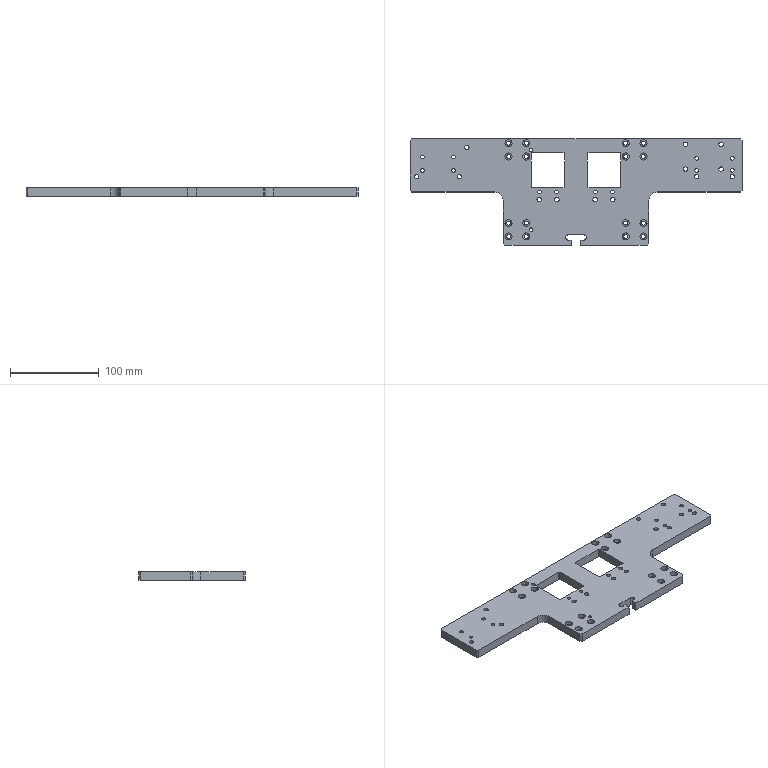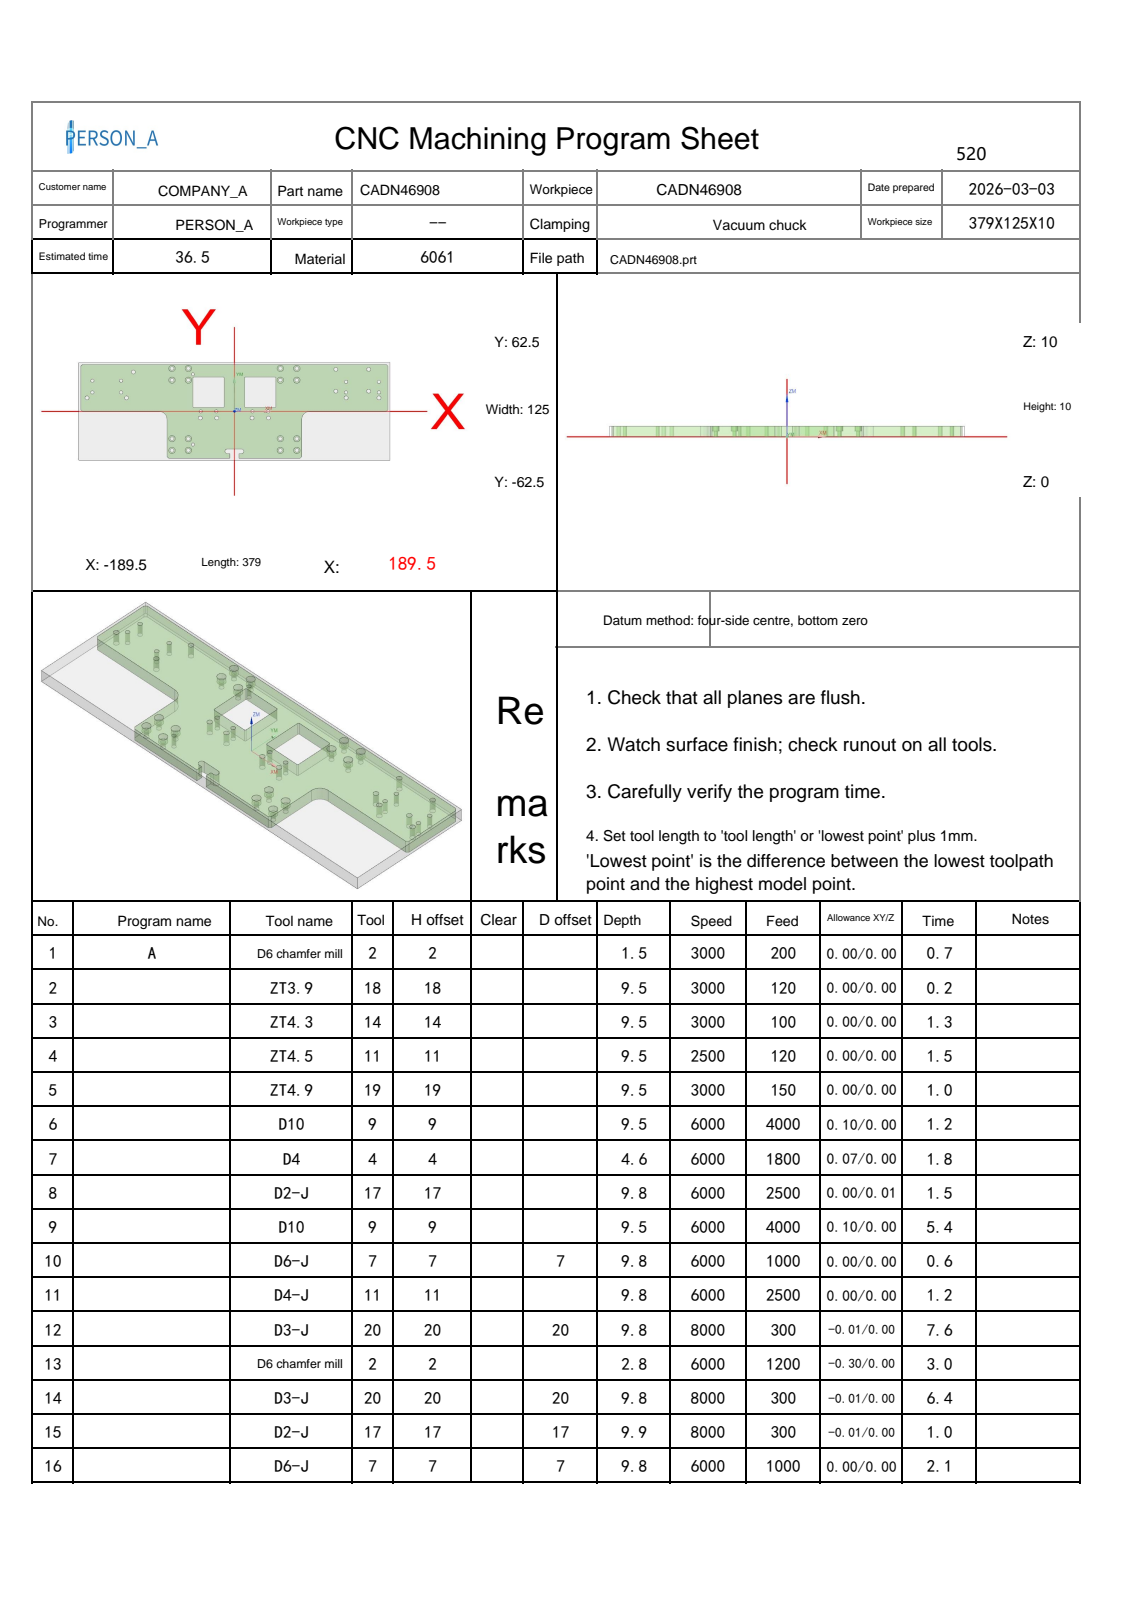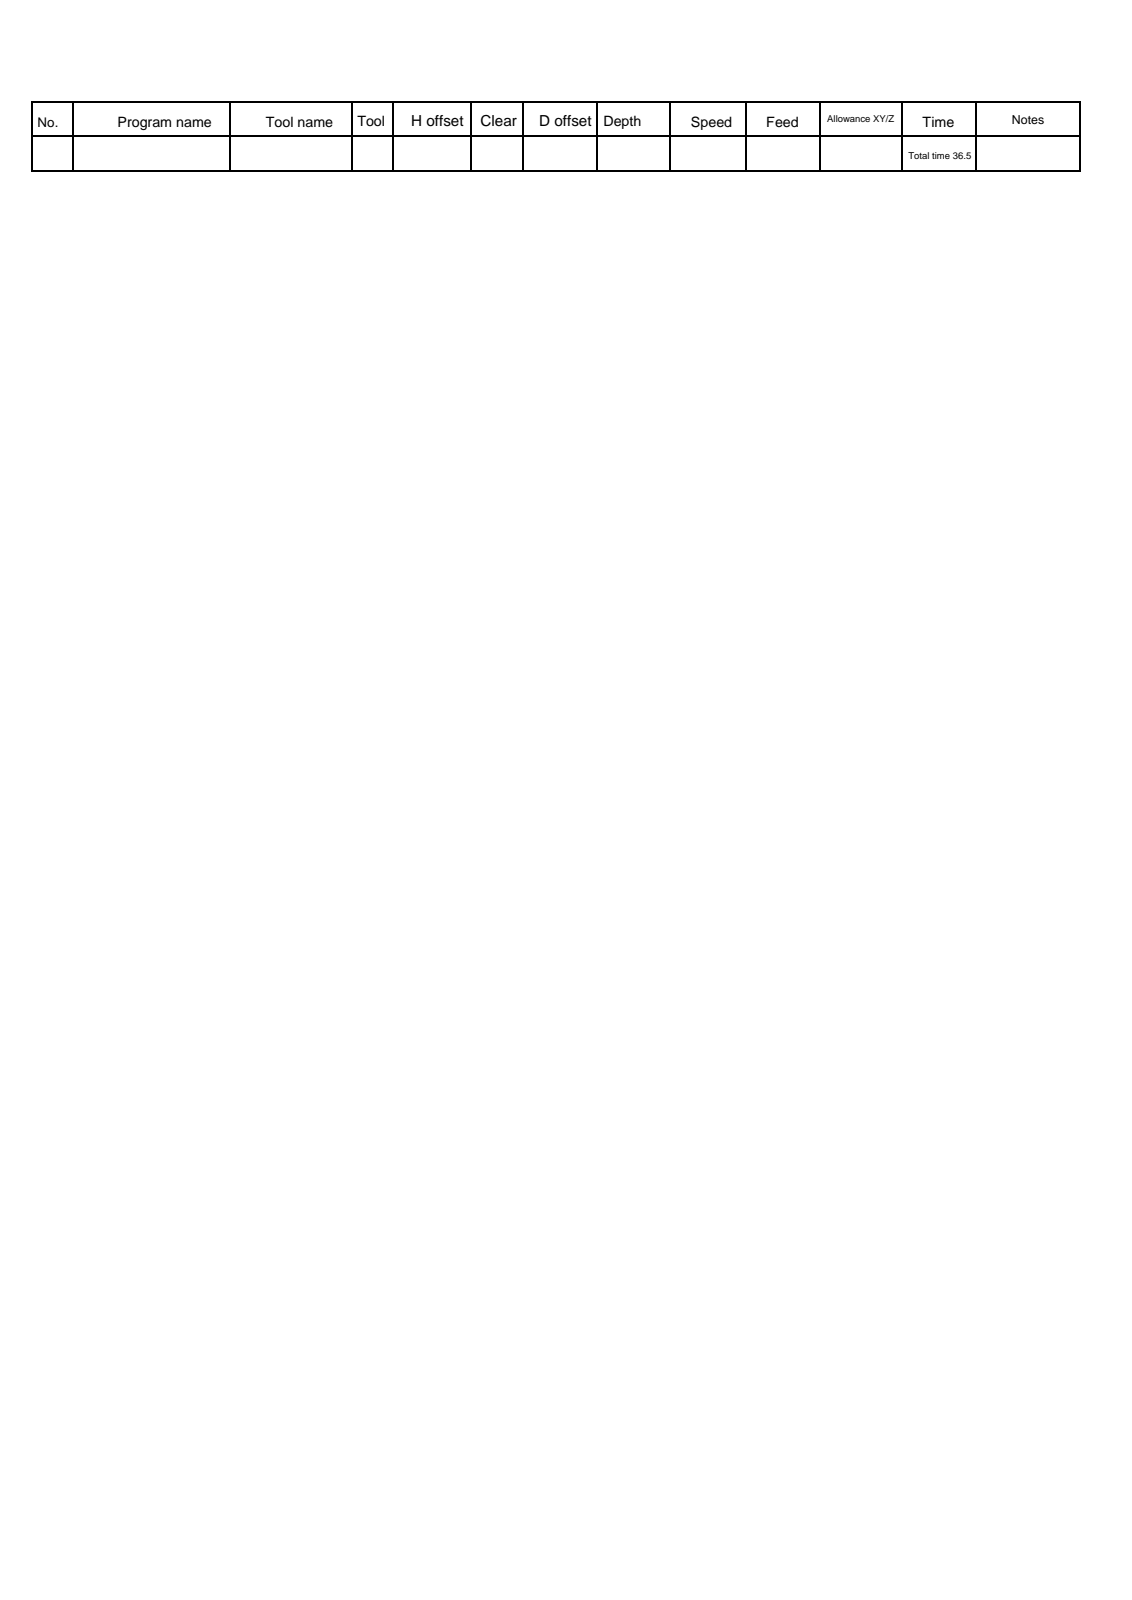NC program | NX | posted by the shop | part box 374 x 120 x 10 mm
Lines 6179 to 7020 of 15301:
N9 T09 M06
(D10  D=10. R=0. H=09 ce=0.10 di=0.00)
G00 G90 G54 X0.0 Y65.1 M03 S6000
G43 H09 Z40.
M08
Z10.5
G01 X185. Z10.41 F4000.
G02 X188.606 Y63.606 Z10.408 I0.0 J-5.1
G01 X190.606 Y61.606 Z10.406
G02 X192.1 Y58. Z10.404 I-3.606 J-3.606
G01 Y2. Z10.377
G02 X190.606 Y-1.606 Z10.375 I-5.1 J0.0
G01 X188.606 Y-3.606 Z10.374
G02 X185. Y-5.1 Z10.372 I-3.606 J3.606
G01 X92. Z10.326
G03 X87.1 Y-10. Z10.323 I0.0 J-4.9
G01 Y-58. Z10.299
G02 X85.606 Y-61.606 Z10.297 I-5.1 J0.0
G01 X83.606 Y-63.606 Z10.296
G02 X80. Y-65.1 Z10.294 I-3.606 J3.606
G01 X5.5 Z10.257
G02 X.4 Y-60. Z10.254 I0.0 J5.1
G01 Y-54.2 Z10.251
G02 X.48 Y-53.3 Z10.25 I5.1 J0.0
G01 X-.48
G02 X-.4 Y-54.2 Z10.249 I-5.02 J-.9
G01 Y-60. Z10.246
G02 X-5.5 Y-65.1 Z10.243 I-5.1 J0.0
G01 X-80. Z10.206
G02 X-83.606 Y-63.606 Z10.204 I0.0 J5.1
G01 X-85.606 Y-61.606 Z10.203
G02 X-87.1 Y-58. Z10.201 I3.606 J3.606
G01 Y-10. Z10.177
G03 X-92. Y-5.1 Z10.174 I-4.9 J0.0
G01 X-185. Z10.128
G02 X-188.606 Y-3.606 Z10.126 I0.0 J5.1
G01 X-190.606 Y-1.606 Z10.125
G02 X-192.1 Y2. Z10.123 I3.606 J3.606
G01 Y58. Z10.096
G02 X-190.606 Y61.606 Z10.094 I5.1 J0.0
G01 X-188.606 Y63.606 Z10.092
G02 X-185. Y65.1 Z10.09 I3.606 J-3.606
G01 X185. Z9.91
G02 X188.606 Y63.606 Z9.908 I0.0 J-5.1
G01 X190.606 Y61.606 Z9.906
G02 X192.1 Y58. Z9.904 I-3.606 J-3.606
G01 Y2. Z9.877
G02 X190.606 Y-1.606 Z9.875 I-5.1 J0.0
G01 X188.606 Y-3.606 Z9.874
G02 X185. Y-5.1 Z9.872 I-3.606 J3.606
G01 X92. Z9.826
G03 X87.1 Y-10. Z9.823 I0.0 J-4.9
G01 Y-58. Z9.799
G02 X85.606 Y-61.606 Z9.797 I-5.1 J0.0
G01 X83.606 Y-63.606 Z9.796
G02 X80. Y-65.1 Z9.794 I-3.606 J3.606
G01 X5.5 Z9.757
G02 X.4 Y-60. Z9.754 I0.0 J5.1
G01 Y-54.2 Z9.751
G02 X.48 Y-53.3 Z9.75 I5.1 J0.0
G01 X-.48
G02 X-.4 Y-54.2 Z9.749 I-5.02 J-.9
G01 Y-60. Z9.746
G02 X-5.5 Y-65.1 Z9.743 I-5.1 J0.0
G01 X-80. Z9.706
G02 X-83.606 Y-63.606 Z9.704 I0.0 J5.1
G01 X-85.606 Y-61.606 Z9.703
G02 X-87.1 Y-58. Z9.701 I3.606 J3.606
G01 Y-10. Z9.677
G03 X-92. Y-5.1 Z9.674 I-4.9 J0.0
G01 X-185. Z9.628
G02 X-188.606 Y-3.606 Z9.626 I0.0 J5.1
G01 X-190.606 Y-1.606 Z9.625
G02 X-192.1 Y2. Z9.623 I3.606 J3.606
G01 Y58. Z9.596
G02 X-190.606 Y61.606 Z9.594 I5.1 J0.0
G01 X-188.606 Y63.606 Z9.592
G02 X-185. Y65.1 Z9.59 I3.606 J-3.606
G01 X185. Z9.41
G02 X188.606 Y63.606 Z9.408 I0.0 J-5.1
G01 X190.606 Y61.606 Z9.406
G02 X192.1 Y58. Z9.404 I-3.606 J-3.606
G01 Y2. Z9.377
G02 X190.606 Y-1.606 Z9.375 I-5.1 J0.0
G01 X188.606 Y-3.606 Z9.374
G02 X185. Y-5.1 Z9.372 I-3.606 J3.606
G01 X92. Z9.326
G03 X87.1 Y-10. Z9.323 I0.0 J-4.9
G01 Y-58. Z9.299
G02 X85.606 Y-61.606 Z9.297 I-5.1 J0.0
G01 X83.606 Y-63.606 Z9.296
G02 X80. Y-65.1 Z9.294 I-3.606 J3.606
G01 X5.5 Z9.257
G02 X.4 Y-60. Z9.254 I0.0 J5.1
G01 Y-54.2 Z9.251
G02 X.48 Y-53.3 Z9.25 I5.1 J0.0
G01 X-.48
G02 X-.4 Y-54.2 Z9.249 I-5.02 J-.9
G01 Y-60. Z9.246
G02 X-5.5 Y-65.1 Z9.243 I-5.1 J0.0
G01 X-80. Z9.206
G02 X-83.606 Y-63.606 Z9.204 I0.0 J5.1
G01 X-85.606 Y-61.606 Z9.203
G02 X-87.1 Y-58. Z9.201 I3.606 J3.606
G01 Y-10. Z9.177
G03 X-92. Y-5.1 Z9.174 I-4.9 J0.0
G01 X-185. Z9.128
G02 X-188.606 Y-3.606 Z9.126 I0.0 J5.1
G01 X-190.606 Y-1.606 Z9.125
G02 X-192.1 Y2. Z9.123 I3.606 J3.606
G01 Y58. Z9.096
G02 X-190.606 Y61.606 Z9.094 I5.1 J0.0
G01 X-188.606 Y63.606 Z9.092
G02 X-185. Y65.1 Z9.09 I3.606 J-3.606
G01 X185. Z8.91
G02 X188.606 Y63.606 Z8.908 I0.0 J-5.1
G01 X190.606 Y61.606 Z8.906
G02 X192.1 Y58. Z8.904 I-3.606 J-3.606
G01 Y2. Z8.877
G02 X190.606 Y-1.606 Z8.875 I-5.1 J0.0
G01 X188.606 Y-3.606 Z8.874
G02 X185. Y-5.1 Z8.872 I-3.606 J3.606
G01 X92. Z8.826
G03 X87.1 Y-10. Z8.823 I0.0 J-4.9
G01 Y-58. Z8.799
G02 X85.606 Y-61.606 Z8.797 I-5.1 J0.0
G01 X83.606 Y-63.606 Z8.796
G02 X80. Y-65.1 Z8.794 I-3.606 J3.606
G01 X5.5 Z8.757
G02 X.4 Y-60. Z8.754 I0.0 J5.1
G01 Y-54.2 Z8.751
G02 X.48 Y-53.3 Z8.75 I5.1 J0.0
G01 X-.48
G02 X-.4 Y-54.2 Z8.749 I-5.02 J-.9
G01 Y-60. Z8.746
G02 X-5.5 Y-65.1 Z8.743 I-5.1 J0.0
G01 X-80. Z8.706
G02 X-83.606 Y-63.606 Z8.704 I0.0 J5.1
G01 X-85.606 Y-61.606 Z8.703
G02 X-87.1 Y-58. Z8.701 I3.606 J3.606
G01 Y-10. Z8.677
G03 X-92. Y-5.1 Z8.674 I-4.9 J0.0
G01 X-185. Z8.628
G02 X-188.606 Y-3.606 Z8.626 I0.0 J5.1
G01 X-190.606 Y-1.606 Z8.625
G02 X-192.1 Y2. Z8.623 I3.606 J3.606
G01 Y58. Z8.596
G02 X-190.606 Y61.606 Z8.594 I5.1 J0.0
G01 X-188.606 Y63.606 Z8.592
G02 X-185. Y65.1 Z8.59 I3.606 J-3.606
G01 X185. Z8.41
G02 X188.606 Y63.606 Z8.408 I0.0 J-5.1
G01 X190.606 Y61.606 Z8.406
G02 X192.1 Y58. Z8.404 I-3.606 J-3.606
G01 Y2. Z8.377
G02 X190.606 Y-1.606 Z8.375 I-5.1 J0.0
G01 X188.606 Y-3.606 Z8.374
G02 X185. Y-5.1 Z8.372 I-3.606 J3.606
G01 X92. Z8.326
G03 X87.1 Y-10. Z8.323 I0.0 J-4.9
G01 Y-58. Z8.299
G02 X85.606 Y-61.606 Z8.297 I-5.1 J0.0
G01 X83.606 Y-63.606 Z8.296
G02 X80. Y-65.1 Z8.294 I-3.606 J3.606
G01 X5.5 Z8.257
G02 X.4 Y-60. Z8.254 I0.0 J5.1
G01 Y-54.2 Z8.251
G02 X.48 Y-53.3 Z8.25 I5.1 J0.0
G01 X-.48
G02 X-.4 Y-54.2 Z8.249 I-5.02 J-.9
G01 Y-60. Z8.246
G02 X-5.5 Y-65.1 Z8.243 I-5.1 J0.0
G01 X-80. Z8.206
G02 X-83.606 Y-63.606 Z8.204 I0.0 J5.1
G01 X-85.606 Y-61.606 Z8.203
G02 X-87.1 Y-58. Z8.201 I3.606 J3.606
G01 Y-10. Z8.177
G03 X-92. Y-5.1 Z8.174 I-4.9 J0.0
G01 X-185. Z8.128
G02 X-188.606 Y-3.606 Z8.126 I0.0 J5.1
G01 X-190.606 Y-1.606 Z8.125
G02 X-192.1 Y2. Z8.123 I3.606 J3.606
G01 Y58. Z8.096
G02 X-190.606 Y61.606 Z8.094 I5.1 J0.0
G01 X-188.606 Y63.606 Z8.092
G02 X-185. Y65.1 Z8.09 I3.606 J-3.606
G01 X185. Z7.91
G02 X188.606 Y63.606 Z7.908 I0.0 J-5.1
G01 X190.606 Y61.606 Z7.906
G02 X192.1 Y58. Z7.904 I-3.606 J-3.606
G01 Y2. Z7.877
G02 X190.606 Y-1.606 Z7.875 I-5.1 J0.0
G01 X188.606 Y-3.606 Z7.874
G02 X185. Y-5.1 Z7.872 I-3.606 J3.606
G01 X92. Z7.826
G03 X87.1 Y-10. Z7.823 I0.0 J-4.9
G01 Y-58. Z7.799
G02 X85.606 Y-61.606 Z7.797 I-5.1 J0.0
G01 X83.606 Y-63.606 Z7.796
G02 X80. Y-65.1 Z7.794 I-3.606 J3.606
G01 X5.5 Z7.757
G02 X.4 Y-60. Z7.754 I0.0 J5.1
G01 Y-54.2 Z7.751
G02 X.48 Y-53.3 Z7.75 I5.1 J0.0
G01 X-.48
G02 X-.4 Y-54.2 Z7.749 I-5.02 J-.9
G01 Y-60. Z7.746
G02 X-5.5 Y-65.1 Z7.743 I-5.1 J0.0
G01 X-80. Z7.706
G02 X-83.606 Y-63.606 Z7.704 I0.0 J5.1
G01 X-85.606 Y-61.606 Z7.703
G02 X-87.1 Y-58. Z7.701 I3.606 J3.606
G01 Y-10. Z7.677
G03 X-92. Y-5.1 Z7.674 I-4.9 J0.0
G01 X-185. Z7.628
G02 X-188.606 Y-3.606 Z7.626 I0.0 J5.1
G01 X-190.606 Y-1.606 Z7.625
G02 X-192.1 Y2. Z7.623 I3.606 J3.606
G01 Y58. Z7.596
G02 X-190.606 Y61.606 Z7.594 I5.1 J0.0
G01 X-188.606 Y63.606 Z7.592
G02 X-185. Y65.1 Z7.59 I3.606 J-3.606
G01 X185. Z7.41
G02 X188.606 Y63.606 Z7.408 I0.0 J-5.1
G01 X190.606 Y61.606 Z7.406
G02 X192.1 Y58. Z7.404 I-3.606 J-3.606
G01 Y2. Z7.377
G02 X190.606 Y-1.606 Z7.375 I-5.1 J0.0
G01 X188.606 Y-3.606 Z7.374
G02 X185. Y-5.1 Z7.372 I-3.606 J3.606
G01 X92. Z7.326
G03 X87.1 Y-10. Z7.323 I0.0 J-4.9
G01 Y-58. Z7.299
G02 X85.606 Y-61.606 Z7.297 I-5.1 J0.0
G01 X83.606 Y-63.606 Z7.296
G02 X80. Y-65.1 Z7.294 I-3.606 J3.606
G01 X5.5 Z7.257
G02 X.4 Y-60. Z7.254 I0.0 J5.1
G01 Y-54.2 Z7.251
G02 X.48 Y-53.3 Z7.25 I5.1 J0.0
G01 X-.48
G02 X-.4 Y-54.2 Z7.249 I-5.02 J-.9
G01 Y-60. Z7.246
G02 X-5.5 Y-65.1 Z7.243 I-5.1 J0.0
G01 X-80. Z7.206
G02 X-83.606 Y-63.606 Z7.204 I0.0 J5.1
G01 X-85.606 Y-61.606 Z7.203
G02 X-87.1 Y-58. Z7.201 I3.606 J3.606
G01 Y-10. Z7.177
G03 X-92. Y-5.1 Z7.174 I-4.9 J0.0
G01 X-185. Z7.128
G02 X-188.606 Y-3.606 Z7.126 I0.0 J5.1
G01 X-190.606 Y-1.606 Z7.125
G02 X-192.1 Y2. Z7.123 I3.606 J3.606
G01 Y58. Z7.096
G02 X-190.606 Y61.606 Z7.094 I5.1 J0.0
G01 X-188.606 Y63.606 Z7.092
G02 X-185. Y65.1 Z7.09 I3.606 J-3.606
G01 X185. Z6.91
G02 X188.606 Y63.606 Z6.908 I0.0 J-5.1
G01 X190.606 Y61.606 Z6.906
G02 X192.1 Y58. Z6.904 I-3.606 J-3.606
G01 Y2. Z6.877
G02 X190.606 Y-1.606 Z6.875 I-5.1 J0.0
G01 X188.606 Y-3.606 Z6.874
G02 X185. Y-5.1 Z6.872 I-3.606 J3.606
G01 X92. Z6.826
G03 X87.1 Y-10. Z6.823 I0.0 J-4.9
G01 Y-58. Z6.799
G02 X85.606 Y-61.606 Z6.797 I-5.1 J0.0
G01 X83.606 Y-63.606 Z6.796
G02 X80. Y-65.1 Z6.794 I-3.606 J3.606
G01 X5.5 Z6.757
G02 X.4 Y-60. Z6.754 I0.0 J5.1
G01 Y-54.2 Z6.751
G02 X.48 Y-53.3 Z6.75 I5.1 J0.0
G01 X-.48
G02 X-.4 Y-54.2 Z6.749 I-5.02 J-.9
G01 Y-60. Z6.746
G02 X-5.5 Y-65.1 Z6.743 I-5.1 J0.0
G01 X-80. Z6.706
G02 X-83.606 Y-63.606 Z6.704 I0.0 J5.1
G01 X-85.606 Y-61.606 Z6.703
G02 X-87.1 Y-58. Z6.701 I3.606 J3.606
G01 Y-10. Z6.677
G03 X-92. Y-5.1 Z6.674 I-4.9 J0.0
G01 X-185. Z6.628
G02 X-188.606 Y-3.606 Z6.626 I0.0 J5.1
G01 X-190.606 Y-1.606 Z6.625
G02 X-192.1 Y2. Z6.623 I3.606 J3.606
G01 Y58. Z6.596
G02 X-190.606 Y61.606 Z6.594 I5.1 J0.0
G01 X-188.606 Y63.606 Z6.592
G02 X-185. Y65.1 Z6.59 I3.606 J-3.606
G01 X185. Z6.41
G02 X188.606 Y63.606 Z6.408 I0.0 J-5.1
G01 X190.606 Y61.606 Z6.406
G02 X192.1 Y58. Z6.404 I-3.606 J-3.606
G01 Y2. Z6.377
G02 X190.606 Y-1.606 Z6.375 I-5.1 J0.0
G01 X188.606 Y-3.606 Z6.374
G02 X185. Y-5.1 Z6.372 I-3.606 J3.606
G01 X92. Z6.326
G03 X87.1 Y-10. Z6.323 I0.0 J-4.9
G01 Y-58. Z6.299
G02 X85.606 Y-61.606 Z6.297 I-5.1 J0.0
G01 X83.606 Y-63.606 Z6.296
G02 X80. Y-65.1 Z6.294 I-3.606 J3.606
G01 X5.5 Z6.257
G02 X.4 Y-60. Z6.254 I0.0 J5.1
G01 Y-54.2 Z6.251
G02 X.48 Y-53.3 Z6.25 I5.1 J0.0
G01 X-.48
G02 X-.4 Y-54.2 Z6.249 I-5.02 J-.9
G01 Y-60. Z6.246
G02 X-5.5 Y-65.1 Z6.243 I-5.1 J0.0
G01 X-80. Z6.206
G02 X-83.606 Y-63.606 Z6.204 I0.0 J5.1
G01 X-85.606 Y-61.606 Z6.203
G02 X-87.1 Y-58. Z6.201 I3.606 J3.606
G01 Y-10. Z6.177
G03 X-92. Y-5.1 Z6.174 I-4.9 J0.0
G01 X-185. Z6.128
G02 X-188.606 Y-3.606 Z6.126 I0.0 J5.1
G01 X-190.606 Y-1.606 Z6.125
G02 X-192.1 Y2. Z6.123 I3.606 J3.606
G01 Y58. Z6.096
G02 X-190.606 Y61.606 Z6.094 I5.1 J0.0
G01 X-188.606 Y63.606 Z6.092
G02 X-185. Y65.1 Z6.09 I3.606 J-3.606
G01 X185. Z5.91
G02 X188.606 Y63.606 Z5.908 I0.0 J-5.1
G01 X190.606 Y61.606 Z5.906
G02 X192.1 Y58. Z5.904 I-3.606 J-3.606
G01 Y2. Z5.877
G02 X190.606 Y-1.606 Z5.875 I-5.1 J0.0
G01 X188.606 Y-3.606 Z5.874
G02 X185. Y-5.1 Z5.872 I-3.606 J3.606
G01 X92. Z5.826
G03 X87.1 Y-10. Z5.823 I0.0 J-4.9
G01 Y-58. Z5.799
G02 X85.606 Y-61.606 Z5.797 I-5.1 J0.0
G01 X83.606 Y-63.606 Z5.796
G02 X80. Y-65.1 Z5.794 I-3.606 J3.606
G01 X5.5 Z5.757
G02 X.4 Y-60. Z5.754 I0.0 J5.1
G01 Y-54.2 Z5.751
G02 X.48 Y-53.3 Z5.75 I5.1 J0.0
G01 X-.48
G02 X-.4 Y-54.2 Z5.749 I-5.02 J-.9
G01 Y-60. Z5.746
G02 X-5.5 Y-65.1 Z5.743 I-5.1 J0.0
G01 X-80. Z5.706
G02 X-83.606 Y-63.606 Z5.704 I0.0 J5.1
G01 X-85.606 Y-61.606 Z5.703
G02 X-87.1 Y-58. Z5.701 I3.606 J3.606
G01 Y-10. Z5.677
G03 X-92. Y-5.1 Z5.674 I-4.9 J0.0
G01 X-185. Z5.628
G02 X-188.606 Y-3.606 Z5.626 I0.0 J5.1
G01 X-190.606 Y-1.606 Z5.625
G02 X-192.1 Y2. Z5.623 I3.606 J3.606
G01 Y58. Z5.596
G02 X-190.606 Y61.606 Z5.594 I5.1 J0.0
G01 X-188.606 Y63.606 Z5.592
G02 X-185. Y65.1 Z5.59 I3.606 J-3.606
G01 X185. Z5.41
G02 X188.606 Y63.606 Z5.408 I0.0 J-5.1
G01 X190.606 Y61.606 Z5.406
G02 X192.1 Y58. Z5.404 I-3.606 J-3.606
G01 Y2. Z5.377
G02 X190.606 Y-1.606 Z5.375 I-5.1 J0.0
G01 X188.606 Y-3.606 Z5.374
G02 X185. Y-5.1 Z5.372 I-3.606 J3.606
G01 X92. Z5.326
G03 X87.1 Y-10. Z5.323 I0.0 J-4.9
G01 Y-58. Z5.299
G02 X85.606 Y-61.606 Z5.297 I-5.1 J0.0
G01 X83.606 Y-63.606 Z5.296
G02 X80. Y-65.1 Z5.294 I-3.606 J3.606
G01 X5.5 Z5.257
G02 X.4 Y-60. Z5.254 I0.0 J5.1
G01 Y-54.2 Z5.251
G02 X.48 Y-53.3 Z5.25 I5.1 J0.0
G01 X-.48
G02 X-.4 Y-54.2 Z5.249 I-5.02 J-.9
G01 Y-60. Z5.246
G02 X-5.5 Y-65.1 Z5.243 I-5.1 J0.0
G01 X-80. Z5.206
G02 X-83.606 Y-63.606 Z5.204 I0.0 J5.1
G01 X-85.606 Y-61.606 Z5.203
G02 X-87.1 Y-58. Z5.201 I3.606 J3.606
G01 Y-10. Z5.177
G03 X-92. Y-5.1 Z5.174 I-4.9 J0.0
G01 X-185. Z5.128
G02 X-188.606 Y-3.606 Z5.126 I0.0 J5.1
G01 X-190.606 Y-1.606 Z5.125
G02 X-192.1 Y2. Z5.123 I3.606 J3.606
G01 Y58. Z5.096
G02 X-190.606 Y61.606 Z5.094 I5.1 J0.0
G01 X-188.606 Y63.606 Z5.092
G02 X-185. Y65.1 Z5.09 I3.606 J-3.606
G01 X185. Z4.91
G02 X188.606 Y63.606 Z4.908 I0.0 J-5.1
G01 X190.606 Y61.606 Z4.906
G02 X192.1 Y58. Z4.904 I-3.606 J-3.606
G01 Y2. Z4.877
G02 X190.606 Y-1.606 Z4.875 I-5.1 J0.0
G01 X188.606 Y-3.606 Z4.874
G02 X185. Y-5.1 Z4.872 I-3.606 J3.606
G01 X92. Z4.826
G03 X87.1 Y-10. Z4.823 I0.0 J-4.9
G01 Y-58. Z4.799
G02 X85.606 Y-61.606 Z4.797 I-5.1 J0.0
G01 X83.606 Y-63.606 Z4.796
G02 X80. Y-65.1 Z4.794 I-3.606 J3.606
G01 X5.5 Z4.757
G02 X.4 Y-60. Z4.754 I0.0 J5.1
G01 Y-54.2 Z4.751
G02 X.48 Y-53.3 Z4.75 I5.1 J0.0
G01 X-.48
G02 X-.4 Y-54.2 Z4.749 I-5.02 J-.9
G01 Y-60. Z4.746
G02 X-5.5 Y-65.1 Z4.743 I-5.1 J0.0
G01 X-80. Z4.706
G02 X-83.606 Y-63.606 Z4.704 I0.0 J5.1
G01 X-85.606 Y-61.606 Z4.703
G02 X-87.1 Y-58. Z4.701 I3.606 J3.606
G01 Y-10. Z4.677
G03 X-92. Y-5.1 Z4.674 I-4.9 J0.0
G01 X-185. Z4.628
G02 X-188.606 Y-3.606 Z4.626 I0.0 J5.1
G01 X-190.606 Y-1.606 Z4.625
G02 X-192.1 Y2. Z4.623 I3.606 J3.606
G01 Y58. Z4.596
G02 X-190.606 Y61.606 Z4.594 I5.1 J0.0
G01 X-188.606 Y63.606 Z4.592
G02 X-185. Y65.1 Z4.59 I3.606 J-3.606
G01 X185. Z4.41
G02 X188.606 Y63.606 Z4.408 I0.0 J-5.1
G01 X190.606 Y61.606 Z4.406
G02 X192.1 Y58. Z4.404 I-3.606 J-3.606
G01 Y2. Z4.377
G02 X190.606 Y-1.606 Z4.375 I-5.1 J0.0
G01 X188.606 Y-3.606 Z4.374
G02 X185. Y-5.1 Z4.372 I-3.606 J3.606
G01 X92. Z4.326
G03 X87.1 Y-10. Z4.323 I0.0 J-4.9
G01 Y-58. Z4.299
G02 X85.606 Y-61.606 Z4.297 I-5.1 J0.0
G01 X83.606 Y-63.606 Z4.296
G02 X80. Y-65.1 Z4.294 I-3.606 J3.606
G01 X5.5 Z4.257
G02 X.4 Y-60. Z4.254 I0.0 J5.1
G01 Y-54.2 Z4.251
G02 X.48 Y-53.3 Z4.25 I5.1 J0.0
G01 X-.48
G02 X-.4 Y-54.2 Z4.249 I-5.02 J-.9
G01 Y-60. Z4.246
G02 X-5.5 Y-65.1 Z4.243 I-5.1 J0.0
G01 X-80. Z4.206
G02 X-83.606 Y-63.606 Z4.204 I0.0 J5.1
G01 X-85.606 Y-61.606 Z4.203
G02 X-87.1 Y-58. Z4.201 I3.606 J3.606
G01 Y-10. Z4.177
G03 X-92. Y-5.1 Z4.174 I-4.9 J0.0
G01 X-185. Z4.128
G02 X-188.606 Y-3.606 Z4.126 I0.0 J5.1
G01 X-190.606 Y-1.606 Z4.125
G02 X-192.1 Y2. Z4.123 I3.606 J3.606
G01 Y58. Z4.096
G02 X-190.606 Y61.606 Z4.094 I5.1 J0.0
G01 X-188.606 Y63.606 Z4.092
G02 X-185. Y65.1 Z4.09 I3.606 J-3.606
G01 X185. Z3.91
G02 X188.606 Y63.606 Z3.908 I0.0 J-5.1
G01 X190.606 Y61.606 Z3.906
G02 X192.1 Y58. Z3.904 I-3.606 J-3.606
G01 Y2. Z3.877
G02 X190.606 Y-1.606 Z3.875 I-5.1 J0.0
G01 X188.606 Y-3.606 Z3.874
G02 X185. Y-5.1 Z3.872 I-3.606 J3.606
G01 X92. Z3.826
G03 X87.1 Y-10. Z3.823 I0.0 J-4.9
G01 Y-58. Z3.799
G02 X85.606 Y-61.606 Z3.797 I-5.1 J0.0
G01 X83.606 Y-63.606 Z3.796
G02 X80. Y-65.1 Z3.794 I-3.606 J3.606
G01 X5.5 Z3.757
G02 X.4 Y-60. Z3.754 I0.0 J5.1
G01 Y-54.2 Z3.751
G02 X.48 Y-53.3 Z3.75 I5.1 J0.0
G01 X-.48
G02 X-.4 Y-54.2 Z3.749 I-5.02 J-.9
G01 Y-60. Z3.746
G02 X-5.5 Y-65.1 Z3.743 I-5.1 J0.0
G01 X-80. Z3.706
G02 X-83.606 Y-63.606 Z3.704 I0.0 J5.1
G01 X-85.606 Y-61.606 Z3.703
G02 X-87.1 Y-58. Z3.701 I3.606 J3.606
G01 Y-10. Z3.677
G03 X-92. Y-5.1 Z3.674 I-4.9 J0.0
G01 X-185. Z3.628
G02 X-188.606 Y-3.606 Z3.626 I0.0 J5.1
G01 X-190.606 Y-1.606 Z3.625
G02 X-192.1 Y2. Z3.623 I3.606 J3.606
G01 Y58. Z3.596
G02 X-190.606 Y61.606 Z3.594 I5.1 J0.0
G01 X-188.606 Y63.606 Z3.592
G02 X-185. Y65.1 Z3.59 I3.606 J-3.606
G01 X185. Z3.41
G02 X188.606 Y63.606 Z3.408 I0.0 J-5.1
G01 X190.606 Y61.606 Z3.406
G02 X192.1 Y58. Z3.404 I-3.606 J-3.606
G01 Y2. Z3.377
G02 X190.606 Y-1.606 Z3.375 I-5.1 J0.0
G01 X188.606 Y-3.606 Z3.374
G02 X185. Y-5.1 Z3.372 I-3.606 J3.606
G01 X92. Z3.326
G03 X87.1 Y-10. Z3.323 I0.0 J-4.9
G01 Y-58. Z3.299
G02 X85.606 Y-61.606 Z3.297 I-5.1 J0.0
G01 X83.606 Y-63.606 Z3.296
G02 X80. Y-65.1 Z3.294 I-3.606 J3.606
G01 X5.5 Z3.257
G02 X.4 Y-60. Z3.254 I0.0 J5.1
G01 Y-54.2 Z3.251
G02 X.48 Y-53.3 Z3.25 I5.1 J0.0
G01 X-.48
G02 X-.4 Y-54.2 Z3.249 I-5.02 J-.9
G01 Y-60. Z3.246
G02 X-5.5 Y-65.1 Z3.243 I-5.1 J0.0
G01 X-80. Z3.206
G02 X-83.606 Y-63.606 Z3.204 I0.0 J5.1
G01 X-85.606 Y-61.606 Z3.203
G02 X-87.1 Y-58. Z3.201 I3.606 J3.606
G01 Y-10. Z3.177
G03 X-92. Y-5.1 Z3.174 I-4.9 J0.0
G01 X-185. Z3.128
G02 X-188.606 Y-3.606 Z3.126 I0.0 J5.1
G01 X-190.606 Y-1.606 Z3.125
G02 X-192.1 Y2. Z3.123 I3.606 J3.606
G01 Y58. Z3.096
G02 X-190.606 Y61.606 Z3.094 I5.1 J0.0
G01 X-188.606 Y63.606 Z3.092
G02 X-185. Y65.1 Z3.09 I3.606 J-3.606
G01 X185. Z2.91
G02 X188.606 Y63.606 Z2.908 I0.0 J-5.1
G01 X190.606 Y61.606 Z2.906
G02 X192.1 Y58. Z2.904 I-3.606 J-3.606
G01 Y2. Z2.877
G02 X190.606 Y-1.606 Z2.875 I-5.1 J0.0
G01 X188.606 Y-3.606 Z2.874
G02 X185. Y-5.1 Z2.872 I-3.606 J3.606
G01 X92. Z2.826
G03 X87.1 Y-10. Z2.823 I0.0 J-4.9
G01 Y-58. Z2.799
G02 X85.606 Y-61.606 Z2.797 I-5.1 J0.0
G01 X83.606 Y-63.606 Z2.796
G02 X80. Y-65.1 Z2.794 I-3.606 J3.606
G01 X5.5 Z2.757
G02 X.4 Y-60. Z2.754 I0.0 J5.1
G01 Y-54.2 Z2.751
G02 X.48 Y-53.3 Z2.75 I5.1 J0.0
G01 X-.48
G02 X-.4 Y-54.2 Z2.749 I-5.02 J-.9
G01 Y-60. Z2.746
G02 X-5.5 Y-65.1 Z2.743 I-5.1 J0.0
G01 X-80. Z2.706
G02 X-83.606 Y-63.606 Z2.704 I0.0 J5.1
G01 X-85.606 Y-61.606 Z2.703
G02 X-87.1 Y-58. Z2.701 I3.606 J3.606
G01 Y-10. Z2.677
G03 X-92. Y-5.1 Z2.674 I-4.9 J0.0
G01 X-185. Z2.628
G02 X-188.606 Y-3.606 Z2.626 I0.0 J5.1
G01 X-190.606 Y-1.606 Z2.625
G02 X-192.1 Y2. Z2.623 I3.606 J3.606
G01 Y58. Z2.596
G02 X-190.606 Y61.606 Z2.594 I5.1 J0.0
G01 X-188.606 Y63.606 Z2.592
G02 X-185. Y65.1 Z2.59 I3.606 J-3.606
G01 X185. Z2.41
G02 X188.606 Y63.606 Z2.408 I0.0 J-5.1
G01 X190.606 Y61.606 Z2.406
G02 X192.1 Y58. Z2.404 I-3.606 J-3.606
G01 Y2. Z2.377
G02 X190.606 Y-1.606 Z2.375 I-5.1 J0.0
G01 X188.606 Y-3.606 Z2.374
G02 X185. Y-5.1 Z2.372 I-3.606 J3.606
G01 X92. Z2.326
G03 X87.1 Y-10. Z2.323 I0.0 J-4.9
G01 Y-58. Z2.299
G02 X85.606 Y-61.606 Z2.297 I-5.1 J0.0
G01 X83.606 Y-63.606 Z2.296
G02 X80. Y-65.1 Z2.294 I-3.606 J3.606
G01 X5.5 Z2.257
G02 X.4 Y-60. Z2.254 I0.0 J5.1
G01 Y-54.2 Z2.251
G02 X.48 Y-53.3 Z2.25 I5.1 J0.0
G01 X-.48
G02 X-.4 Y-54.2 Z2.249 I-5.02 J-.9
G01 Y-60. Z2.246
G02 X-5.5 Y-65.1 Z2.243 I-5.1 J0.0
G01 X-80. Z2.206
G02 X-83.606 Y-63.606 Z2.204 I0.0 J5.1
G01 X-85.606 Y-61.606 Z2.203
G02 X-87.1 Y-58. Z2.201 I3.606 J3.606
G01 Y-10. Z2.177
G03 X-92. Y-5.1 Z2.174 I-4.9 J0.0
G01 X-185. Z2.128
G02 X-188.606 Y-3.606 Z2.126 I0.0 J5.1
G01 X-190.606 Y-1.606 Z2.125
G02 X-192.1 Y2. Z2.123 I3.606 J3.606
G01 Y58. Z2.096
G02 X-190.606 Y61.606 Z2.094 I5.1 J0.0
G01 X-188.606 Y63.606 Z2.092
G02 X-185. Y65.1 Z2.09 I3.606 J-3.606
G01 X185. Z1.91
G02 X188.606 Y63.606 Z1.908 I0.0 J-5.1
G01 X190.606 Y61.606 Z1.906
G02 X192.1 Y58. Z1.904 I-3.606 J-3.606
G01 Y2. Z1.877
G02 X190.606 Y-1.606 Z1.875 I-5.1 J0.0
G01 X188.606 Y-3.606 Z1.874
G02 X185. Y-5.1 Z1.872 I-3.606 J3.606
G01 X92. Z1.826
G03 X87.1 Y-10. Z1.823 I0.0 J-4.9
G01 Y-58. Z1.799
G02 X85.606 Y-61.606 Z1.797 I-5.1 J0.0
G01 X83.606 Y-63.606 Z1.796
G02 X80. Y-65.1 Z1.794 I-3.606 J3.606
G01 X5.5 Z1.757
G02 X.4 Y-60. Z1.754 I0.0 J5.1
G01 Y-54.2 Z1.751
G02 X.48 Y-53.3 Z1.75 I5.1 J0.0
G01 X-.48
G02 X-.4 Y-54.2 Z1.749 I-5.02 J-.9
G01 Y-60. Z1.746
G02 X-5.5 Y-65.1 Z1.743 I-5.1 J0.0
G01 X-80. Z1.706
G02 X-83.606 Y-63.606 Z1.704 I0.0 J5.1
G01 X-85.606 Y-61.606 Z1.703
G02 X-87.1 Y-58. Z1.701 I3.606 J3.606
G01 Y-10. Z1.677
G03 X-92. Y-5.1 Z1.674 I-4.9 J0.0
G01 X-185. Z1.628
G02 X-188.606 Y-3.606 Z1.626 I0.0 J5.1
G01 X-190.606 Y-1.606 Z1.625
G02 X-192.1 Y2. Z1.623 I3.606 J3.606
G01 Y58. Z1.596
G02 X-190.606 Y61.606 Z1.594 I5.1 J0.0
G01 X-188.606 Y63.606 Z1.592
G02 X-185. Y65.1 Z1.59 I3.606 J-3.606
G01 X185. Z1.41
G02 X188.606 Y63.606 Z1.408 I0.0 J-5.1
G01 X190.606 Y61.606 Z1.406
G02 X192.1 Y58. Z1.404 I-3.606 J-3.606
G01 Y2. Z1.377
G02 X190.606 Y-1.606 Z1.375 I-5.1 J0.0
G01 X188.606 Y-3.606 Z1.374
G02 X185. Y-5.1 Z1.372 I-3.606 J3.606
G01 X92. Z1.326
G03 X87.1 Y-10. Z1.323 I0.0 J-4.9
G01 Y-58. Z1.299
G02 X85.606 Y-61.606 Z1.297 I-5.1 J0.0
G01 X83.606 Y-63.606 Z1.296
G02 X80. Y-65.1 Z1.294 I-3.606 J3.606
G01 X5.5 Z1.257
G02 X.4 Y-60. Z1.254 I0.0 J5.1
G01 Y-54.2 Z1.251
G02 X.48 Y-53.3 Z1.25 I5.1 J0.0
G01 X-.48
G02 X-.4 Y-54.2 Z1.249 I-5.02 J-.9
G01 Y-60. Z1.246
G02 X-5.5 Y-65.1 Z1.243 I-5.1 J0.0
G01 X-80. Z1.206
G02 X-83.606 Y-63.606 Z1.204 I0.0 J5.1
G01 X-85.606 Y-61.606 Z1.203
G02 X-87.1 Y-58. Z1.201 I3.606 J3.606
G01 Y-10. Z1.177
G03 X-92. Y-5.1 Z1.174 I-4.9 J0.0
G01 X-185. Z1.128
G02 X-188.606 Y-3.606 Z1.126 I0.0 J5.1
G01 X-190.606 Y-1.606 Z1.125
G02 X-192.1 Y2. Z1.123 I3.606 J3.606
G01 Y58. Z1.096
G02 X-190.606 Y61.606 Z1.094 I5.1 J0.0
G01 X-188.606 Y63.606 Z1.092
G02 X-185. Y65.1 Z1.09 I3.606 J-3.606
G01 X185. Z.91
G02 X188.606 Y63.606 Z.908 I0.0 J-5.1
G01 X190.606 Y61.606 Z.906
G02 X192.1 Y58. Z.904 I-3.606 J-3.606
G01 Y2. Z.877
G02 X190.606 Y-1.606 Z.875 I-5.1 J0.0
G01 X188.606 Y-3.606 Z.874
G02 X185. Y-5.1 Z.872 I-3.606 J3.606
G01 X92. Z.826
G03 X87.1 Y-10. Z.823 I0.0 J-4.9
G01 Y-58. Z.799
G02 X85.606 Y-61.606 Z.797 I-5.1 J0.0
G01 X83.606 Y-63.606 Z.796
G02 X80. Y-65.1 Z.794 I-3.606 J3.606
G01 X5.5 Z.757
G02 X.4 Y-60. Z.754 I0.0 J5.1
G01 Y-54.2 Z.751
G02 X.48 Y-53.3 Z.75 I5.1 J0.0
G01 X-.48
G02 X-.4 Y-54.2 Z.749 I-5.02 J-.9
G01 Y-60. Z.746
G02 X-5.5 Y-65.1 Z.743 I-5.1 J0.0
G01 X-80. Z.706
G02 X-83.606 Y-63.606 Z.704 I0.0 J5.1
G01 X-85.606 Y-61.606 Z.703
G02 X-87.1 Y-58. Z.701 I3.606 J3.606
G01 Y-10. Z.677
G03 X-92. Y-5.1 Z.674 I-4.9 J0.0
G01 X-185. Z.628
G02 X-188.606 Y-3.606 Z.626 I0.0 J5.1
G01 X-190.606 Y-1.606 Z.625
G02 X-192.1 Y2. Z.623 I3.606 J3.606
G01 Y58. Z.596
G02 X-190.606 Y61.606 Z.594 I5.1 J0.0
G01 X-188.606 Y63.606 Z.592
G02 X-185. Y65.1 Z.59 I3.606 J-3.606
G01 X0.0 Z.5
X185.
G02 X188.606 Y63.606 I0.0 J-5.1
G01 X190.606 Y61.606
G02 X192.1 Y58. I-3.606 J-3.606
G01 Y2.
G02 X190.606 Y-1.606 I-5.1 J0.0
G01 X188.606 Y-3.606
G02 X185. Y-5.1 I-3.606 J3.606
G01 X92.
G03 X87.1 Y-10. I0.0 J-4.9
G01 Y-58.
G02 X85.606 Y-61.606 I-5.1 J0.0
G01 X83.606 Y-63.606
G02 X80. Y-65.1 I-3.606 J3.606
G01 X5.5
G02 X.4 Y-60. I0.0 J5.1
G01 Y-54.2
G02 X.48 Y-53.3 I5.1 J0.0
G01 X-.48
G02 X-.4 Y-54.2 I-5.02 J-.9
G01 Y-60.
G02 X-5.5 Y-65.1 I-5.1 J0.0
G01 X-80.
G02 X-83.606 Y-63.606 I0.0 J5.1
G01 X-85.606 Y-61.606
G02 X-87.1 Y-58. I3.606 J3.606
G01 Y-10.
G03 X-92. Y-5.1 I-4.9 J0.0
G01 X-185.
G02 X-188.606 Y-3.606 I0.0 J5.1
G01 X-190.606 Y-1.606
G02 X-192.1 Y2. I3.606 J3.606
G01 Y58.
G02 X-190.606 Y61.606 I5.1 J0.0
G01 X-188.606 Y63.606
G02 X-185. Y65.1 I3.606 J-3.606
G01 X0.0
X.5
Z1.5
G00 Z40.
G91 G28 Z0.0
M05
M09
G91 G28 Z0.0
M01
N10 T07 M06
(D6-J  D=6. R=0. H=07 ce=0.00 di=0.00)
G00 G90 G54 X-16.7 Y40. M03 S6000
G43 H07 Z40.
M08
Z1.
G01 Z.5 F1000.
G41 D07
X-16.5
G03 X-15.5 Y41. I0.0 J1.
G01 X-47.5
Y8.
X-15.5
Y41.
X-16.
G03 X-17. Y40. I0.0 J-1.
G01 G40 Y39.8
Z1.
G00 Z40.
X46.3 Y40.
Z1.
G01 Z.5
G41 D07
X46.5
G03 X47.5 Y41. I0.0 J1.
G01 X15.5
Y8.
X47.5
Y41.
X47.
G03 X46. Y40. I0.0 J-1.
G01 G40 Y39.8
Z1.
G00 Z40.
G00 G90 X-16.6 Y40. M03 S6000
Z40.
Z.7
G01 Z.2 F1000.
G41 D07
X-16.5
G03 X-15.5 Y41. I0.0 J1.
G01 X-47.5
Y8.
X-15.5
Y41.
X-16.
G03 X-17. Y40. I0.0 J-1.
G01 G40 Y39.9
Z.7
G00 Z40.
X46.4 Y40.
Z.7
G01 Z.2
G41 D07
X46.5
G03 X47.5 Y41. I0.0 J1.
G01 X15.5
Y8.
X47.5
Y41.
X47.
G03 X46. Y40. I0.0 J-1.
G01 G40 Y39.9
Z.7
G00 Z40.
G91 G28 Z0.0
M05
M09
G91 G28 Z0.0
M01